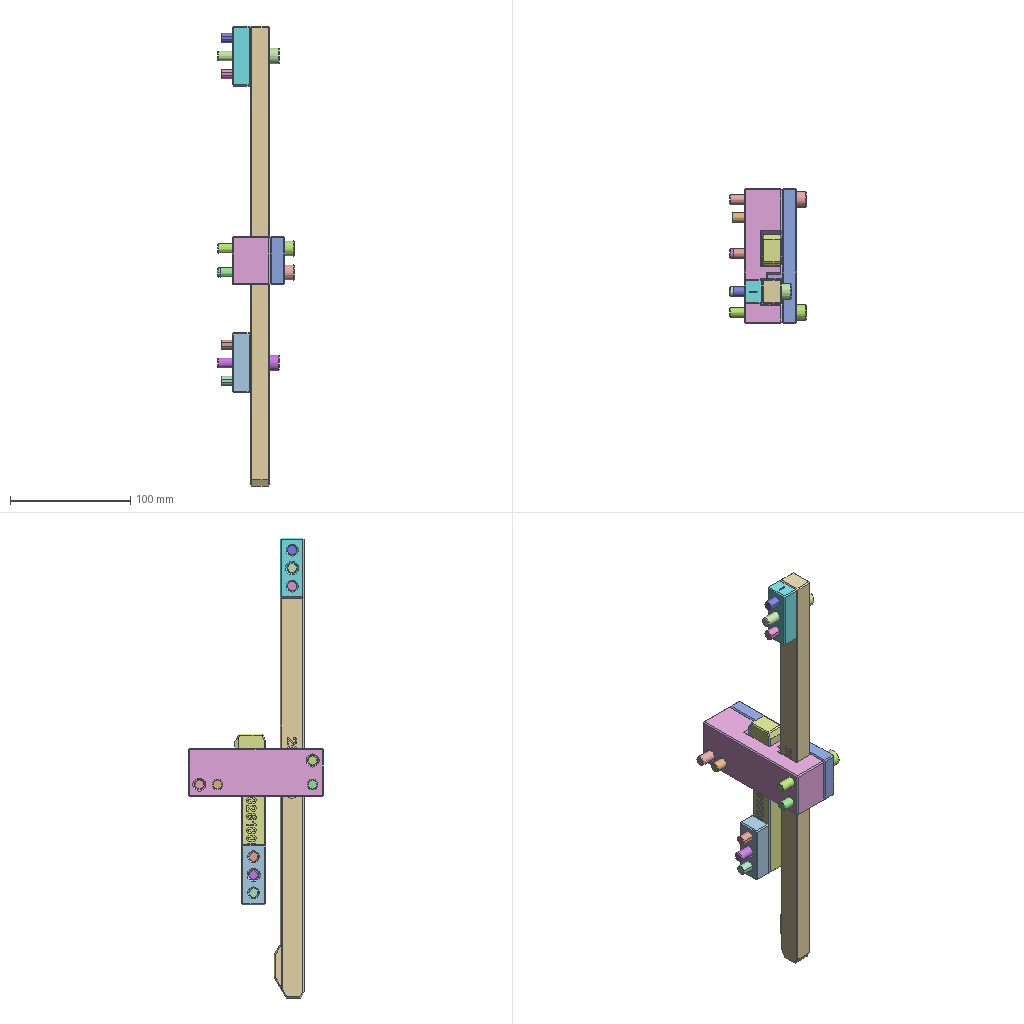Assembly | NX | 22 different items | 22 placed | box 64 x 112 x 382 mm
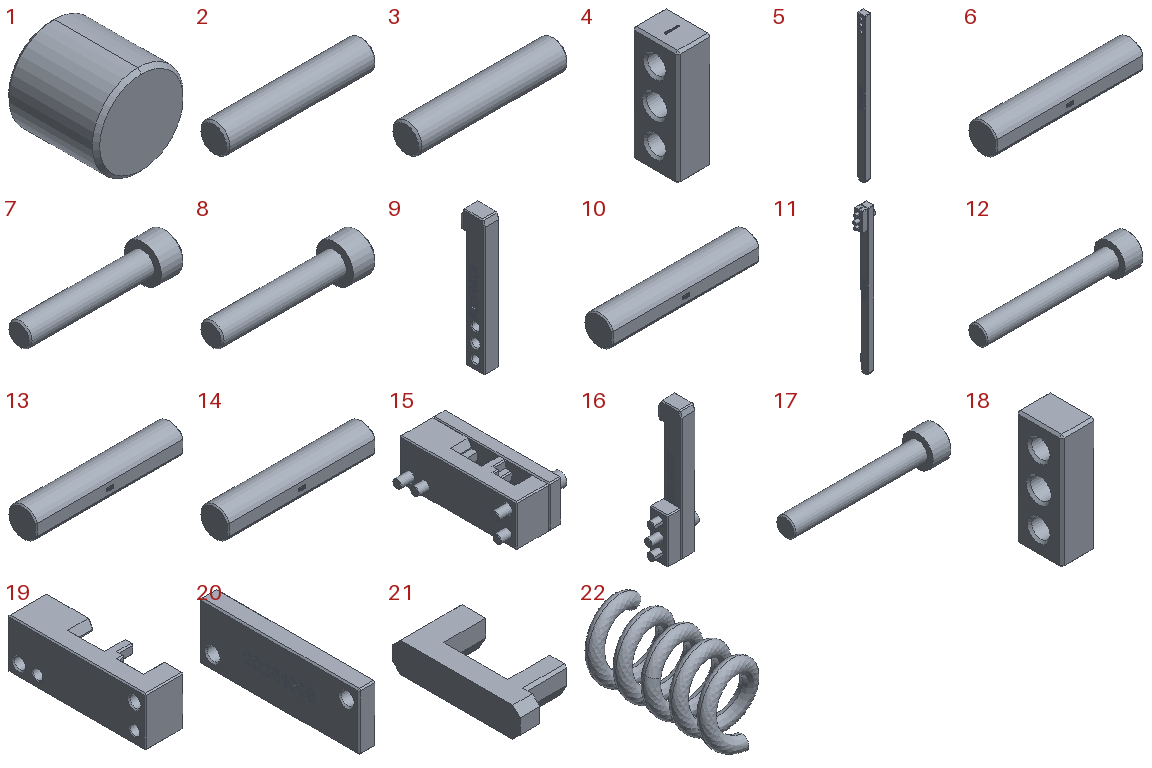Parts list (item | quantity | parent item | size | volume | features):
1 | x1 | in 15 | 12 x 12 x 12 mm | 1208 mm3 | features solid 2
2 | x1 | in 15 | 41 x 8 x 8 mm | 2055 mm3 | features solid 2
3 | x1 | in 15 | 41 x 8 x 8 mm | 2055 mm3 | features solid 2
4 | x1 | in 11 | 15 x 20 x 50 mm | 12288 mm3 | features BREP 8, solid 2, CHAMFER 1, SUBTRACT 1
5 | x1 | in 11 | 16 x 25 x 382.34 mm | 118829 mm3 | features BREP 8, CHAMFER 2, solid 2, SUBTRACT 1
6 | x1 | in 11 | 40 x 7.7 x 8 mm | 1857 mm3 | features BREP 2, solid 2, SUBTRACT 1
7 | x1 | in 11 | 51 x 13 x 13 mm | 3079 mm3 | features CHAMFER 6, BREP 2, solid 2, SUBTRACT 1
8 | x1 | in 16 | 51 x 13 x 13 mm | 3079 mm3 | features CHAMFER 6, BREP 2, solid 2, SUBTRACT 1
9 | x1 | in 16 | 16 x 25.5 x 142 mm | 43802 mm3 | features BREP 8, CHAMFER 2, solid 2, SUBTRACT 1
10 | x1 | in 16 | 40 x 7.7 x 8 mm | 1857 mm3 | features BREP 2, solid 2, SUBTRACT 1
11 | x1 | - | 51 x 25 x 382.34 mm | 137909 mm3 | features BREP 22, solid 10, CHAMFER 9, SUBTRACT 5
12 | x1 | in 15 | 63.5 x 13 x 13 mm | 3707 mm3 | features CHAMFER 6, BREP 2, solid 2, SUBTRACT 1
13 | x1 | in 11 | 40 x 7.7 x 8 mm | 1857 mm3 | features BREP 2, solid 2, SUBTRACT 1
14 | x1 | in 16 | 40 x 7.7 x 8 mm | 1857 mm3 | features BREP 2, solid 2, SUBTRACT 1
15 | x1 | - | 63.5 x 112 x 40 mm | 159871 mm3 | features BREP 20, solid 18, CHAMFER 16, SUBTRACT 4
16 | x1 | - | 51 x 25.5 x 142 mm | 62882 mm3 | features BREP 22, solid 10, CHAMFER 9, SUBTRACT 5
17 | x1 | in 15 | 63.5 x 13 x 13 mm | 3707 mm3 | features CHAMFER 6, BREP 2, solid 2, SUBTRACT 1
18 | x1 | in 16 | 15 x 20 x 50 mm | 12288 mm3 | features BREP 8, solid 2, CHAMFER 1, SUBTRACT 1
19 | x1 | in 15 | 31.5 x 112 x 40 mm | 86589 mm3 | features BREP 8, CHAMFER 2, solid 2, SUBTRACT 1
20 | x1 | in 15 | 12 x 112 x 40 mm | 51813 mm3 | features BREP 8, CHAMFER 2, solid 2, SUBTRACT 1
21 | x1 | in 15 | 25 x 51.5 x 12 mm | 8371 mm3 | features solid 2
22 | x1 | in 15 | 10 x 20.499 x 10 mm | 364.957 mm3 | features solid 2